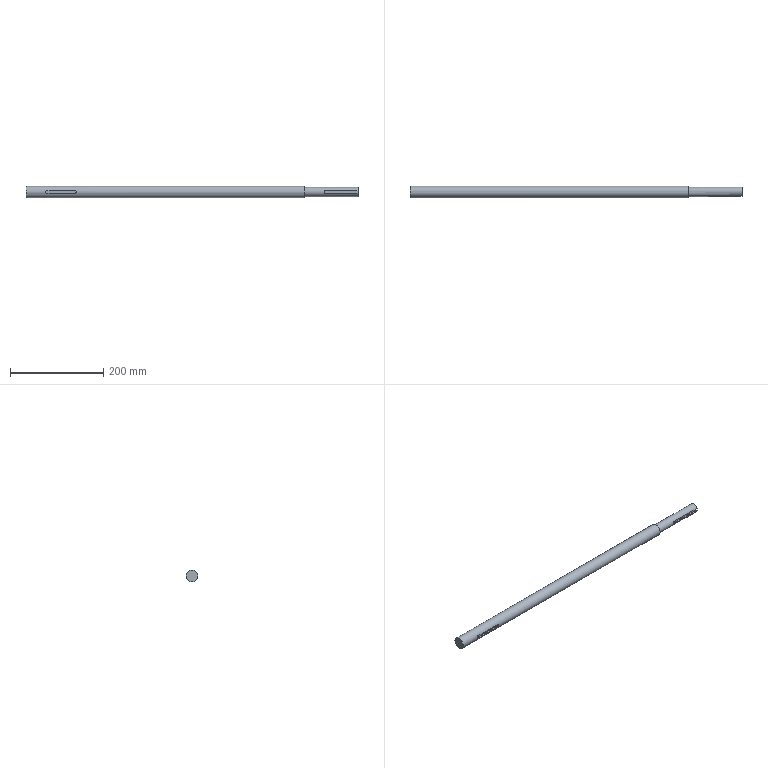Part | STEP file | shaftfor roller511 | 1 solid | 16 faces | box 713 x 25 x 25 mm | volume 326518 mm3 | plane 9 | cylinder 5 | spline 2 | commonest cylinder face diameters 6 x3 20 x1 25 x1